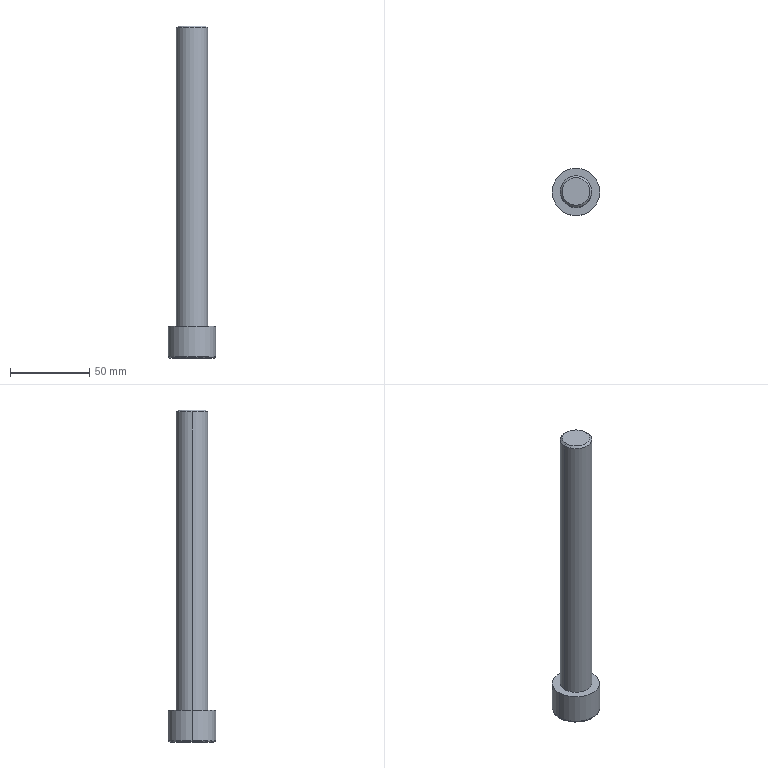Part | Creo | 1 solid | 20 faces | box 30 x 30 x 210 mm | volume 70457 mm3 | plane 10 | cylinder 4 | torus 4 | cone 2 | commonest cylinder face diameters 20 x2 30 x2
STEP:
#1=CARTESIAN_POINT('',(-275.,275.,-95.75));
#2=VERTEX_POINT('',#1);
#3=CARTESIAN_POINT('',(-255.,275.,-95.75));
#4=VERTEX_POINT('',#3);
#5=CARTESIAN_POINT('',(-265.,275.,-95.75));
#6=DIRECTION('',(0.,0.,1.));
#7=DIRECTION('',(-1.,0.,0.));
#8=AXIS2_PLACEMENT_3D('',#5,#6,#7);
#9=CIRCLE('',#8,10.);
#10=EDGE_CURVE('',#2,#4,#9,.T.);
#11=ORIENTED_EDGE('',*,*,#10,.T.);
#12=CARTESIAN_POINT('',(-255.,275.,-284.5));
#13=VERTEX_POINT('',#12);
#14=CARTESIAN_POINT('',(-255.,275.,-284.5));
#15=DIRECTION('',(0.,0.,1.));
#16=VECTOR('',#15,188.75);
#17=LINE('',#14,#16);
#18=EDGE_CURVE('',#13,#4,#17,.T.);
#19=ORIENTED_EDGE('',*,*,#18,.F.);
#20=CARTESIAN_POINT('',(-275.,275.,-284.5));
#21=VERTEX_POINT('',#20);
#22=CARTESIAN_POINT('',(-265.,275.,-284.5));
#23=DIRECTION('',(0.,0.,-1.));
#24=DIRECTION('',(1.,0.,0.));
#25=AXIS2_PLACEMENT_3D('',#22,#23,#24);
#26=CIRCLE('',#25,10.);
#27=EDGE_CURVE('',#13,#21,#26,.T.);
#28=ORIENTED_EDGE('',*,*,#27,.T.);
#29=CARTESIAN_POINT('',(-275.,275.,-284.5));
#30=DIRECTION('',(0.,0.,1.));
#31=VECTOR('',#30,188.75);
#32=LINE('',#29,#31);
#33=EDGE_CURVE('',#21,#2,#32,.T.);
#34=ORIENTED_EDGE('',*,*,#33,.T.);
#35=EDGE_LOOP('',(#11,#19,#28,#34));
#36=FACE_OUTER_BOUND('',#35,.F.);
#37=CARTESIAN_POINT('',(-265.,275.,-284.5));
#38=DIRECTION('',(0.,0.,1.));
#39=DIRECTION('',(-1.,0.,0.));
#40=AXIS2_PLACEMENT_3D('',#37,#38,#39);
#41=CYLINDRICAL_SURFACE('',#40,10.);
#42=ADVANCED_FACE('',(#36),#41,.T.);
#43=CARTESIAN_POINT('',(-273.75,275.,-94.5));
#44=VERTEX_POINT('',#43);
#45=CARTESIAN_POINT('',(-256.25,275.,-94.5));
#46=VERTEX_POINT('',#45);
#47=CARTESIAN_POINT('',(-265.,275.,-94.5));
#48=DIRECTION('',(0.,0.,1.));
#49=DIRECTION('',(-1.,0.,0.));
#50=AXIS2_PLACEMENT_3D('',#47,#48,#49);
#51=CIRCLE('',#50,8.75);
#52=EDGE_CURVE('',#44,#46,#51,.T.);
#53=ORIENTED_EDGE('',*,*,#52,.T.);
#54=CARTESIAN_POINT('',(-256.25,275.,-94.5));
#55=DIRECTION('',(0.7071,0.,-0.7071));
#56=VECTOR('',#55,1.768);
#57=LINE('',#54,#56);
#58=EDGE_CURVE('',#46,#4,#57,.T.);
#59=ORIENTED_EDGE('',*,*,#58,.T.);
#60=ORIENTED_EDGE('',*,*,#10,.F.);
#61=CARTESIAN_POINT('',(-273.75,275.,-94.5));
#62=DIRECTION('',(-0.7071,0.,-0.7071));
#63=VECTOR('',#62,1.768);
#64=LINE('',#61,#63);
#65=EDGE_CURVE('',#44,#2,#64,.T.);
#66=ORIENTED_EDGE('',*,*,#65,.F.);
#67=EDGE_LOOP('',(#53,#59,#60,#66));
#68=FACE_OUTER_BOUND('',#67,.F.);
#69=CARTESIAN_POINT('',(-265.,275.,-95.125));
#70=DIRECTION('',(0.,0.,-1.));
#71=DIRECTION('',(1.,0.,0.));
#72=AXIS2_PLACEMENT_3D('',#69,#70,#71);
#73=CONICAL_SURFACE('',#72,9.375,45.);
#74=ADVANCED_FACE('',(#68),#73,.T.);
#75=CARTESIAN_POINT('',(-265.,275.,-94.5));
#76=DIRECTION('',(0.,0.,1.));
#77=DIRECTION('',(1.,0.,0.));
#78=AXIS2_PLACEMENT_3D('',#75,#76,#77);
#79=CIRCLE('',#78,8.75);
#80=EDGE_CURVE('',#46,#44,#79,.T.);
#81=ORIENTED_EDGE('',*,*,#80,.F.);
#82=ORIENTED_EDGE('',*,*,#52,.F.);
#83=EDGE_LOOP('',(#81,#82));
#84=FACE_OUTER_BOUND('',#83,.F.);
#85=CARTESIAN_POINT('',(-265.,275.,-94.5));
#86=DIRECTION('',(0.,0.,-1.));
#87=DIRECTION('',(1.,0.,0.));
#88=AXIS2_PLACEMENT_3D('',#85,#86,#87);
#89=PLANE('',#88);
#90=ADVANCED_FACE('',(#84),#89,.F.);
#91=ORIENTED_EDGE('',*,*,#80,.T.);
#92=ORIENTED_EDGE('',*,*,#65,.T.);
#93=CARTESIAN_POINT('',(-265.,275.,-95.75));
#94=DIRECTION('',(0.,0.,1.));
#95=DIRECTION('',(1.,0.,0.));
#96=AXIS2_PLACEMENT_3D('',#93,#94,#95);
#97=CIRCLE('',#96,10.);
#98=EDGE_CURVE('',#4,#2,#97,.T.);
#99=ORIENTED_EDGE('',*,*,#98,.F.);
#100=ORIENTED_EDGE('',*,*,#58,.F.);
#101=EDGE_LOOP('',(#91,#92,#99,#100));
#102=FACE_OUTER_BOUND('',#101,.F.);
#103=CARTESIAN_POINT('',(-265.,275.,-95.125));
#104=DIRECTION('',(0.,0.,-1.));
#105=DIRECTION('',(1.,0.,0.));
#106=AXIS2_PLACEMENT_3D('',#103,#104,#105);
#107=CONICAL_SURFACE('',#106,9.375,45.);
#108=ADVANCED_FACE('',(#102),#107,.T.);
#109=ORIENTED_EDGE('',*,*,#98,.T.);
#110=ORIENTED_EDGE('',*,*,#33,.F.);
#111=CARTESIAN_POINT('',(-265.,275.,-284.5));
#112=DIRECTION('',(0.,0.,-1.));
#113=DIRECTION('',(-1.,0.,0.));
#114=AXIS2_PLACEMENT_3D('',#111,#112,#113);
#115=CIRCLE('',#114,10.);
#116=EDGE_CURVE('',#21,#13,#115,.T.);
#117=ORIENTED_EDGE('',*,*,#116,.T.);
#118=ORIENTED_EDGE('',*,*,#18,.T.);
#119=EDGE_LOOP('',(#109,#110,#117,#118));
#120=FACE_OUTER_BOUND('',#119,.F.);
#121=CARTESIAN_POINT('',(-265.,275.,-284.5));
#122=DIRECTION('',(0.,0.,1.));
#123=DIRECTION('',(-1.,0.,0.));
#124=AXIS2_PLACEMENT_3D('',#121,#122,#123);
#125=CYLINDRICAL_SURFACE('',#124,10.);
#126=ADVANCED_FACE('',(#120),#125,.T.);
#127=CARTESIAN_POINT('',(-250.,275.,-284.5));
#128=VERTEX_POINT('',#127);
#129=CARTESIAN_POINT('',(-280.,275.,-284.5));
#130=VERTEX_POINT('',#129);
#131=CARTESIAN_POINT('',(-265.,275.,-284.5));
#132=DIRECTION('',(0.,0.,1.));
#133=DIRECTION('',(1.,0.,0.));
#134=AXIS2_PLACEMENT_3D('',#131,#132,#133);
#135=CIRCLE('',#134,15.);
#136=EDGE_CURVE('',#128,#130,#135,.T.);
#137=ORIENTED_EDGE('',*,*,#136,.F.);
#138=CARTESIAN_POINT('',(-265.,275.,-284.5));
#139=DIRECTION('',(0.,0.,1.));
#140=DIRECTION('',(-1.,0.,0.));
#141=AXIS2_PLACEMENT_3D('',#138,#139,#140);
#142=CIRCLE('',#141,15.);
#143=EDGE_CURVE('',#130,#128,#142,.T.);
#144=ORIENTED_EDGE('',*,*,#143,.F.);
#145=EDGE_LOOP('',(#137,#144));
#146=FACE_OUTER_BOUND('',#145,.F.);
#147=ORIENTED_EDGE('',*,*,#27,.F.);
#148=ORIENTED_EDGE('',*,*,#116,.F.);
#149=EDGE_LOOP('',(#147,#148));
#150=FACE_BOUND('',#149,.F.);
#151=CARTESIAN_POINT('',(-265.,275.,-284.5));
#152=DIRECTION('',(0.,0.,1.));
#153=DIRECTION('',(-1.,0.,0.));
#154=AXIS2_PLACEMENT_3D('',#151,#152,#153);
#155=PLANE('',#154);
#156=ADVANCED_FACE('',(#146,#150),#155,.T.);
#157=CARTESIAN_POINT('',(-280.,275.,-303.5));
#158=VERTEX_POINT('',#157);
#159=CARTESIAN_POINT('',(-250.,275.,-303.5));
#160=VERTEX_POINT('',#159);
#161=CARTESIAN_POINT('',(-265.,275.,-303.5));
#162=DIRECTION('',(0.,0.,-1.));
#163=DIRECTION('',(-1.,0.,0.));
#164=AXIS2_PLACEMENT_3D('',#161,#162,#163);
#165=CIRCLE('',#164,15.);
#166=EDGE_CURVE('',#158,#160,#165,.T.);
#167=ORIENTED_EDGE('',*,*,#166,.T.);
#168=CARTESIAN_POINT('',(-250.,275.,-284.5));
#169=DIRECTION('',(0.,0.,-1.));
#170=VECTOR('',#169,19.);
#171=LINE('',#168,#170);
#172=EDGE_CURVE('',#128,#160,#171,.T.);
#173=ORIENTED_EDGE('',*,*,#172,.F.);
#174=ORIENTED_EDGE('',*,*,#136,.T.);
#175=CARTESIAN_POINT('',(-280.,275.,-284.5));
#176=DIRECTION('',(0.,0.,-1.));
#177=VECTOR('',#176,19.);
#178=LINE('',#175,#177);
#179=EDGE_CURVE('',#130,#158,#178,.T.);
#180=ORIENTED_EDGE('',*,*,#179,.T.);
#181=EDGE_LOOP('',(#167,#173,#174,#180));
#182=FACE_OUTER_BOUND('',#181,.F.);
#183=CARTESIAN_POINT('',(-265.,275.,-284.5));
#184=DIRECTION('',(0.,0.,-1.));
#185=DIRECTION('',(1.,0.,0.));
#186=AXIS2_PLACEMENT_3D('',#183,#184,#185);
#187=CYLINDRICAL_SURFACE('',#186,15.);
#188=ADVANCED_FACE('',(#182),#187,.T.);
#189=ORIENTED_EDGE('',*,*,#166,.F.);
#190=CARTESIAN_POINT('',(-279.707,275.,-304.207));
#191=VERTEX_POINT('',#190);
#192=CARTESIAN_POINT('',(-279.,275.,-303.5));
#193=DIRECTION('',(0.,-1.,0.));
#194=DIRECTION('',(-1.,0.,0.));
#195=AXIS2_PLACEMENT_3D('',#192,#193,#194);
#196=CIRCLE('',#195,1.);
#197=EDGE_CURVE('',#158,#191,#196,.T.);
#198=ORIENTED_EDGE('',*,*,#197,.T.);
#199=CARTESIAN_POINT('',(-250.293,275.,-304.207));
#200=VERTEX_POINT('',#199);
#201=CARTESIAN_POINT('',(-265.,275.,-304.207));
#202=DIRECTION('',(0.,0.,-1.));
#203=DIRECTION('',(-1.,0.,0.));
#204=AXIS2_PLACEMENT_3D('',#201,#202,#203);
#205=CIRCLE('',#204,14.707);
#206=EDGE_CURVE('',#191,#200,#205,.T.);
#207=ORIENTED_EDGE('',*,*,#206,.T.);
#208=CARTESIAN_POINT('',(-251.,275.,-303.5));
#209=DIRECTION('',(0.,1.,0.));
#210=DIRECTION('',(1.,0.,0.));
#211=AXIS2_PLACEMENT_3D('',#208,#209,#210);
#212=CIRCLE('',#211,1.);
#213=EDGE_CURVE('',#160,#200,#212,.T.);
#214=ORIENTED_EDGE('',*,*,#213,.F.);
#215=EDGE_LOOP('',(#189,#198,#207,#214));
#216=FACE_OUTER_BOUND('',#215,.F.);
#217=CARTESIAN_POINT('',(-265.,275.,-303.5));
#218=DIRECTION('',(0.,0.,-1.));
#219=DIRECTION('',(1.,0.,0.));
#220=AXIS2_PLACEMENT_3D('',#217,#218,#219);
#221=TOROIDAL_SURFACE('',#220,14.,1.);
#222=ADVANCED_FACE('',(#216),#221,.T.);
#223=CARTESIAN_POINT('',(-265.,275.,-303.5));
#224=DIRECTION('',(0.,0.,-1.));
#225=DIRECTION('',(1.,0.,0.));
#226=AXIS2_PLACEMENT_3D('',#223,#224,#225);
#227=CIRCLE('',#226,15.);
#228=EDGE_CURVE('',#160,#158,#227,.T.);
#229=ORIENTED_EDGE('',*,*,#228,.F.);
#230=ORIENTED_EDGE('',*,*,#213,.T.);
#231=CARTESIAN_POINT('',(-265.,275.,-304.207));
#232=DIRECTION('',(0.,0.,-1.));
#233=DIRECTION('',(1.,0.,0.));
#234=AXIS2_PLACEMENT_3D('',#231,#232,#233);
#235=CIRCLE('',#234,14.707);
#236=EDGE_CURVE('',#200,#191,#235,.T.);
#237=ORIENTED_EDGE('',*,*,#236,.T.);
#238=ORIENTED_EDGE('',*,*,#197,.F.);
#239=EDGE_LOOP('',(#229,#230,#237,#238));
#240=FACE_OUTER_BOUND('',#239,.F.);
#241=CARTESIAN_POINT('',(-265.,275.,-303.5));
#242=DIRECTION('',(0.,0.,-1.));
#243=DIRECTION('',(1.,0.,0.));
#244=AXIS2_PLACEMENT_3D('',#241,#242,#243);
#245=TOROIDAL_SURFACE('',#244,14.,1.);
#246=ADVANCED_FACE('',(#240),#245,.T.);
#247=ORIENTED_EDGE('',*,*,#228,.T.);
#248=ORIENTED_EDGE('',*,*,#179,.F.);
#249=ORIENTED_EDGE('',*,*,#143,.T.);
#250=ORIENTED_EDGE('',*,*,#172,.T.);
#251=EDGE_LOOP('',(#247,#248,#249,#250));
#252=FACE_OUTER_BOUND('',#251,.F.);
#253=CARTESIAN_POINT('',(-265.,275.,-284.5));
#254=DIRECTION('',(0.,0.,-1.));
#255=DIRECTION('',(1.,0.,0.));
#256=AXIS2_PLACEMENT_3D('',#253,#254,#255);
#257=CYLINDRICAL_SURFACE('',#256,15.);
#258=ADVANCED_FACE('',(#252),#257,.T.);
#259=CARTESIAN_POINT('',(-251.,275.,-304.5));
#260=VERTEX_POINT('',#259);
#261=CARTESIAN_POINT('',(-279.,275.,-304.5));
#262=VERTEX_POINT('',#261);
#263=CARTESIAN_POINT('',(-265.,275.,-304.5));
#264=DIRECTION('',(0.,0.,-1.));
#265=DIRECTION('',(1.,0.,0.));
#266=AXIS2_PLACEMENT_3D('',#263,#264,#265);
#267=CIRCLE('',#266,14.);
#268=EDGE_CURVE('',#260,#262,#267,.T.);
#269=ORIENTED_EDGE('',*,*,#268,.T.);
#270=CARTESIAN_POINT('',(-279.,275.,-303.5));
#271=DIRECTION('',(0.,-1.,0.));
#272=DIRECTION('',(-0.7071,0.,-0.7071));
#273=AXIS2_PLACEMENT_3D('',#270,#271,#272);
#274=CIRCLE('',#273,1.);
#275=EDGE_CURVE('',#191,#262,#274,.T.);
#276=ORIENTED_EDGE('',*,*,#275,.F.);
#277=ORIENTED_EDGE('',*,*,#236,.F.);
#278=CARTESIAN_POINT('',(-251.,275.,-303.5));
#279=DIRECTION('',(0.,1.,0.));
#280=DIRECTION('',(0.7071,0.,-0.7071));
#281=AXIS2_PLACEMENT_3D('',#278,#279,#280);
#282=CIRCLE('',#281,1.);
#283=EDGE_CURVE('',#200,#260,#282,.T.);
#284=ORIENTED_EDGE('',*,*,#283,.T.);
#285=EDGE_LOOP('',(#269,#276,#277,#284));
#286=FACE_OUTER_BOUND('',#285,.F.);
#287=CARTESIAN_POINT('',(-265.,275.,-303.5));
#288=DIRECTION('',(0.,0.,-1.));
#289=DIRECTION('',(1.,0.,0.));
#290=AXIS2_PLACEMENT_3D('',#287,#288,#289);
#291=TOROIDAL_SURFACE('',#290,14.,1.);
#292=ADVANCED_FACE('',(#286),#291,.T.);
#293=ORIENTED_EDGE('',*,*,#268,.F.);
#294=CARTESIAN_POINT('',(-265.,275.,-304.5));
#295=DIRECTION('',(0.,0.,-1.));
#296=DIRECTION('',(-1.,0.,0.));
#297=AXIS2_PLACEMENT_3D('',#294,#295,#296);
#298=CIRCLE('',#297,14.);
#299=EDGE_CURVE('',#262,#260,#298,.T.);
#300=ORIENTED_EDGE('',*,*,#299,.F.);
#301=EDGE_LOOP('',(#293,#300));
#302=FACE_OUTER_BOUND('',#301,.F.);
#303=CARTESIAN_POINT('',(-260.093,283.5,-304.5));
#304=VERTEX_POINT('',#303);
#305=CARTESIAN_POINT('',(-269.907,283.5,-304.5));
#306=VERTEX_POINT('',#305);
#307=CARTESIAN_POINT('',(-260.093,283.5,-304.5));
#308=DIRECTION('',(-1.,0.,0.));
#309=VECTOR('',#308,9.815);
#310=LINE('',#307,#309);
#311=EDGE_CURVE('',#304,#306,#310,.T.);
#312=ORIENTED_EDGE('',*,*,#311,.F.);
#313=CARTESIAN_POINT('',(-255.185,275.,-304.5));
#314=VERTEX_POINT('',#313);
#315=CARTESIAN_POINT('',(-255.185,275.,-304.5));
#316=DIRECTION('',(-0.5,0.866,0.));
#317=VECTOR('',#316,9.815);
#318=LINE('',#315,#317);
#319=EDGE_CURVE('',#314,#304,#318,.T.);
#320=ORIENTED_EDGE('',*,*,#319,.F.);
#321=CARTESIAN_POINT('',(-260.093,266.5,-304.5));
#322=VERTEX_POINT('',#321);
#323=CARTESIAN_POINT('',(-260.093,266.5,-304.5));
#324=DIRECTION('',(0.5,0.866,0.));
#325=VECTOR('',#324,9.815);
#326=LINE('',#323,#325);
#327=EDGE_CURVE('',#322,#314,#326,.T.);
#328=ORIENTED_EDGE('',*,*,#327,.F.);
#329=CARTESIAN_POINT('',(-269.907,266.5,-304.5));
#330=VERTEX_POINT('',#329);
#331=CARTESIAN_POINT('',(-269.907,266.5,-304.5));
#332=DIRECTION('',(1.,0.,0.));
#333=VECTOR('',#332,9.815);
#334=LINE('',#331,#333);
#335=EDGE_CURVE('',#330,#322,#334,.T.);
#336=ORIENTED_EDGE('',*,*,#335,.F.);
#337=CARTESIAN_POINT('',(-274.815,275.,-304.5));
#338=VERTEX_POINT('',#337);
#339=CARTESIAN_POINT('',(-274.815,275.,-304.5));
#340=DIRECTION('',(0.5,-0.866,0.));
#341=VECTOR('',#340,9.815);
#342=LINE('',#339,#341);
#343=EDGE_CURVE('',#338,#330,#342,.T.);
#344=ORIENTED_EDGE('',*,*,#343,.F.);
#345=CARTESIAN_POINT('',(-269.907,283.5,-304.5));
#346=DIRECTION('',(-0.5,-0.866,0.));
#347=VECTOR('',#346,9.815);
#348=LINE('',#345,#347);
#349=EDGE_CURVE('',#306,#338,#348,.T.);
#350=ORIENTED_EDGE('',*,*,#349,.F.);
#351=EDGE_LOOP('',(#312,#320,#328,#336,#344,#350));
#352=FACE_BOUND('',#351,.F.);
#353=CARTESIAN_POINT('',(-265.,275.,-304.5));
#354=DIRECTION('',(0.,0.,-1.));
#355=DIRECTION('',(1.,0.,0.));
#356=AXIS2_PLACEMENT_3D('',#353,#354,#355);
#357=PLANE('',#356);
#358=ADVANCED_FACE('',(#302,#352),#357,.T.);
#359=ORIENTED_EDGE('',*,*,#299,.T.);
#360=ORIENTED_EDGE('',*,*,#283,.F.);
#361=ORIENTED_EDGE('',*,*,#206,.F.);
#362=ORIENTED_EDGE('',*,*,#275,.T.);
#363=EDGE_LOOP('',(#359,#360,#361,#362));
#364=FACE_OUTER_BOUND('',#363,.F.);
#365=CARTESIAN_POINT('',(-265.,275.,-303.5));
#366=DIRECTION('',(0.,0.,-1.));
#367=DIRECTION('',(1.,0.,0.));
#368=AXIS2_PLACEMENT_3D('',#365,#366,#367);
#369=TOROIDAL_SURFACE('',#368,14.,1.);
#370=ADVANCED_FACE('',(#364),#369,.T.);
#371=ORIENTED_EDGE('',*,*,#311,.T.);
#372=CARTESIAN_POINT('',(-269.907,283.5,-291.3));
#373=VERTEX_POINT('',#372);
#374=CARTESIAN_POINT('',(-269.907,283.5,-304.5));
#375=DIRECTION('',(0.,0.,1.));
#376=VECTOR('',#375,13.2);
#377=LINE('',#374,#376);
#378=EDGE_CURVE('',#306,#373,#377,.T.);
#379=ORIENTED_EDGE('',*,*,#378,.T.);
#380=CARTESIAN_POINT('',(-260.093,283.5,-291.3));
#381=VERTEX_POINT('',#380);
#382=CARTESIAN_POINT('',(-260.093,283.5,-291.3));
#383=DIRECTION('',(-1.,0.,0.));
#384=VECTOR('',#383,9.815);
#385=LINE('',#382,#384);
#386=EDGE_CURVE('',#381,#373,#385,.T.);
#387=ORIENTED_EDGE('',*,*,#386,.F.);
#388=CARTESIAN_POINT('',(-260.093,283.5,-304.5));
#389=DIRECTION('',(0.,0.,1.));
#390=VECTOR('',#389,13.2);
#391=LINE('',#388,#390);
#392=EDGE_CURVE('',#304,#381,#391,.T.);
#393=ORIENTED_EDGE('',*,*,#392,.F.);
#394=EDGE_LOOP('',(#371,#379,#387,#393));
#395=FACE_OUTER_BOUND('',#394,.F.);
#396=CARTESIAN_POINT('',(-269.907,283.5,-291.3));
#397=DIRECTION('',(0.,1.,0.));
#398=DIRECTION('',(0.,0.,1.));
#399=AXIS2_PLACEMENT_3D('',#396,#397,#398);
#400=PLANE('',#399);
#401=ADVANCED_FACE('',(#395),#400,.F.);
#402=ORIENTED_EDGE('',*,*,#349,.T.);
#403=CARTESIAN_POINT('',(-274.815,275.,-291.3));
#404=VERTEX_POINT('',#403);
#405=CARTESIAN_POINT('',(-274.815,275.,-304.5));
#406=DIRECTION('',(0.,0.,1.));
#407=VECTOR('',#406,13.2);
#408=LINE('',#405,#407);
#409=EDGE_CURVE('',#338,#404,#408,.T.);
#410=ORIENTED_EDGE('',*,*,#409,.T.);
#411=CARTESIAN_POINT('',(-274.815,275.,-291.3));
#412=DIRECTION('',(0.5,0.866,0.));
#413=VECTOR('',#412,9.815);
#414=LINE('',#411,#413);
#415=EDGE_CURVE('',#404,#373,#414,.T.);
#416=ORIENTED_EDGE('',*,*,#415,.T.);
#417=ORIENTED_EDGE('',*,*,#378,.F.);
#418=EDGE_LOOP('',(#402,#410,#416,#417));
#419=FACE_OUTER_BOUND('',#418,.F.);
#420=CARTESIAN_POINT('',(-274.815,275.,-291.3));
#421=DIRECTION('',(-0.866,0.5,0.));
#422=DIRECTION('',(0.5,0.866,0.));
#423=AXIS2_PLACEMENT_3D('',#420,#421,#422);
#424=PLANE('',#423);
#425=ADVANCED_FACE('',(#419),#424,.F.);
#426=ORIENTED_EDGE('',*,*,#343,.T.);
#427=CARTESIAN_POINT('',(-269.907,266.5,-291.3));
#428=VERTEX_POINT('',#427);
#429=CARTESIAN_POINT('',(-269.907,266.5,-304.5));
#430=DIRECTION('',(0.,0.,1.));
#431=VECTOR('',#430,13.2);
#432=LINE('',#429,#431);
#433=EDGE_CURVE('',#330,#428,#432,.T.);
#434=ORIENTED_EDGE('',*,*,#433,.T.);
#435=CARTESIAN_POINT('',(-269.907,266.5,-291.3));
#436=DIRECTION('',(-0.5,0.866,0.));
#437=VECTOR('',#436,9.815);
#438=LINE('',#435,#437);
#439=EDGE_CURVE('',#428,#404,#438,.T.);
#440=ORIENTED_EDGE('',*,*,#439,.T.);
#441=ORIENTED_EDGE('',*,*,#409,.F.);
#442=EDGE_LOOP('',(#426,#434,#440,#441));
#443=FACE_OUTER_BOUND('',#442,.F.);
#444=CARTESIAN_POINT('',(-269.907,266.5,-291.3));
#445=DIRECTION('',(-0.866,-0.5,0.));
#446=DIRECTION('',(-0.5,0.866,0.));
#447=AXIS2_PLACEMENT_3D('',#444,#445,#446);
#448=PLANE('',#447);
#449=ADVANCED_FACE('',(#443),#448,.F.);
#450=ORIENTED_EDGE('',*,*,#335,.T.);
#451=CARTESIAN_POINT('',(-260.093,266.5,-291.3));
#452=VERTEX_POINT('',#451);
#453=CARTESIAN_POINT('',(-260.093,266.5,-304.5));
#454=DIRECTION('',(0.,0.,1.));
#455=VECTOR('',#454,13.2);
#456=LINE('',#453,#455);
#457=EDGE_CURVE('',#322,#452,#456,.T.);
#458=ORIENTED_EDGE('',*,*,#457,.T.);
#459=CARTESIAN_POINT('',(-269.907,266.5,-291.3));
#460=DIRECTION('',(1.,0.,0.));
#461=VECTOR('',#460,9.815);
#462=LINE('',#459,#461);
#463=EDGE_CURVE('',#428,#452,#462,.T.);
#464=ORIENTED_EDGE('',*,*,#463,.F.);
#465=ORIENTED_EDGE('',*,*,#433,.F.);
#466=EDGE_LOOP('',(#450,#458,#464,#465));
#467=FACE_OUTER_BOUND('',#466,.F.);
#468=CARTESIAN_POINT('',(-260.093,266.5,-291.3));
#469=DIRECTION('',(0.,-1.,0.));
#470=DIRECTION('',(0.,0.,-1.));
#471=AXIS2_PLACEMENT_3D('',#468,#469,#470);
#472=PLANE('',#471);
#473=ADVANCED_FACE('',(#467),#472,.F.);
#474=ORIENTED_EDGE('',*,*,#327,.T.);
#475=CARTESIAN_POINT('',(-255.185,275.,-291.3));
#476=VERTEX_POINT('',#475);
#477=CARTESIAN_POINT('',(-255.185,275.,-304.5));
#478=DIRECTION('',(0.,0.,1.));
#479=VECTOR('',#478,13.2);
#480=LINE('',#477,#479);
#481=EDGE_CURVE('',#314,#476,#480,.T.);
#482=ORIENTED_EDGE('',*,*,#481,.T.);
#483=CARTESIAN_POINT('',(-255.185,275.,-291.3));
#484=DIRECTION('',(-0.5,-0.866,0.));
#485=VECTOR('',#484,9.815);
#486=LINE('',#483,#485);
#487=EDGE_CURVE('',#476,#452,#486,.T.);
#488=ORIENTED_EDGE('',*,*,#487,.T.);
#489=ORIENTED_EDGE('',*,*,#457,.F.);
#490=EDGE_LOOP('',(#474,#482,#488,#489));
#491=FACE_OUTER_BOUND('',#490,.F.);
#492=CARTESIAN_POINT('',(-255.185,275.,-291.3));
#493=DIRECTION('',(0.866,-0.5,0.));
#494=DIRECTION('',(-0.5,-0.866,0.));
#495=AXIS2_PLACEMENT_3D('',#492,#493,#494);
#496=PLANE('',#495);
#497=ADVANCED_FACE('',(#491),#496,.F.);
#498=ORIENTED_EDGE('',*,*,#319,.T.);
#499=ORIENTED_EDGE('',*,*,#392,.T.);
#500=CARTESIAN_POINT('',(-260.093,283.5,-291.3));
#501=DIRECTION('',(0.5,-0.866,0.));
#502=VECTOR('',#501,9.815);
#503=LINE('',#500,#502);
#504=EDGE_CURVE('',#381,#476,#503,.T.);
#505=ORIENTED_EDGE('',*,*,#504,.T.);
#506=ORIENTED_EDGE('',*,*,#481,.F.);
#507=EDGE_LOOP('',(#498,#499,#505,#506));
#508=FACE_OUTER_BOUND('',#507,.F.);
#509=CARTESIAN_POINT('',(-260.093,283.5,-291.3));
#510=DIRECTION('',(0.866,0.5,0.));
#511=DIRECTION('',(0.5,-0.866,0.));
#512=AXIS2_PLACEMENT_3D('',#509,#510,#511);
#513=PLANE('',#512);
#514=ADVANCED_FACE('',(#508),#513,.F.);
#515=ORIENTED_EDGE('',*,*,#386,.T.);
#516=ORIENTED_EDGE('',*,*,#415,.F.);
#517=ORIENTED_EDGE('',*,*,#439,.F.);
#518=ORIENTED_EDGE('',*,*,#463,.T.);
#519=ORIENTED_EDGE('',*,*,#487,.F.);
#520=ORIENTED_EDGE('',*,*,#504,.F.);
#521=EDGE_LOOP('',(#515,#516,#517,#518,#519,#520));
#522=FACE_OUTER_BOUND('',#521,.F.);
#523=CARTESIAN_POINT('',(-260.093,283.5,-291.3));
#524=DIRECTION('',(0.,0.,-1.));
#525=DIRECTION('',(1.,0.,0.));
#526=AXIS2_PLACEMENT_3D('',#523,#524,#525);
#527=PLANE('',#526);
#528=ADVANCED_FACE('',(#522),#527,.T.);
#529=CLOSED_SHELL('',(#42,#74,#90,#108,#126,#156,#188,#222,#246,#258,#292,#358,#370,#401,#425,#449,#473,#497,#514,#528));
#530=MANIFOLD_SOLID_BREP('',#529);
#531=(LENGTH_UNIT()NAMED_UNIT(*)SI_UNIT(.MILLI.,.METRE.));
#532=UNCERTAINTY_MEASURE_WITH_UNIT(LENGTH_MEASURE(0.02142),#531,'','');
#533=(NAMED_UNIT(*)PLANE_ANGLE_UNIT()SI_UNIT($,.RADIAN.));
#534=PLANE_ANGLE_MEASURE_WITH_UNIT(PLANE_ANGLE_MEASURE(0.01745),#533);
#535=(CONVERSION_BASED_UNIT('DEGREE',#534)NAMED_UNIT(*)PLANE_ANGLE_UNIT());
#536=(NAMED_UNIT(*)SI_UNIT($,.STERADIAN.)SOLID_ANGLE_UNIT());
#537=(GEOMETRIC_REPRESENTATION_CONTEXT(3)GLOBAL_UNCERTAINTY_ASSIGNED_CONTEXT((#532))GLOBAL_UNIT_ASSIGNED_CONTEXT((#531,#535,#536))REPRESENTATION_CONTEXT('',''));
#538=ADVANCED_BREP_SHAPE_REPRESENTATION('',(#530),#537);